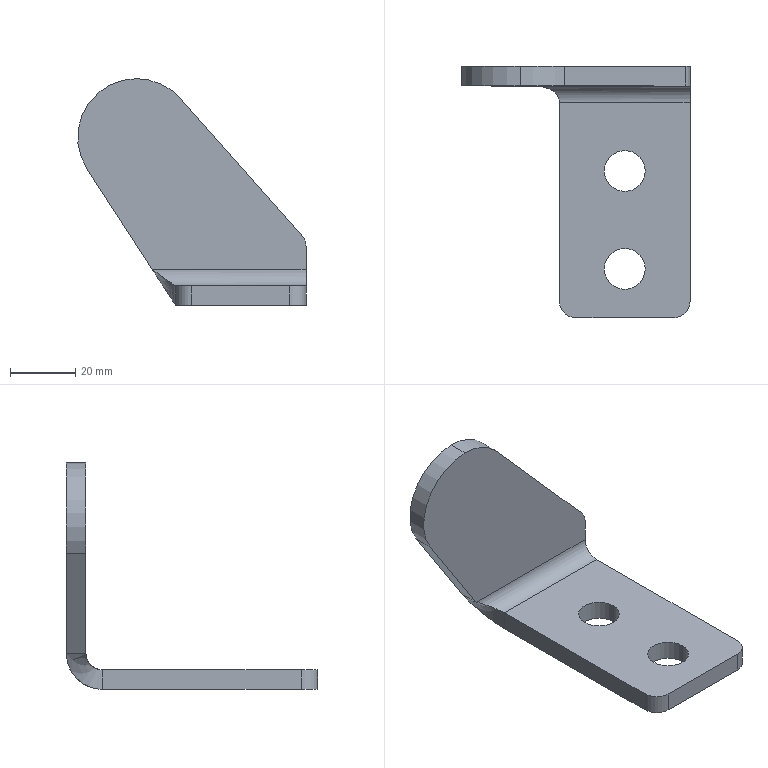Part | SolidWorks | features ICE 2, Fillet 1, FlatPattern 1, SMBaseFlange 1, SheetMetal 1 | 1 solid | 23 faces | box 70 x 77 x 69.5 mm | volume 32666 mm3 | cylinder 11 | plane 11 | spline 1 | commonest cylinder face diameters 10 x4 12.5 x4 36 x2 22 x1
STEP:
#1=CARTESIAN_POINT('',(-52.,71.,69.5));
#2=VERTEX_POINT('',#1);
#3=CARTESIAN_POINT('',(-67.093,71.,41.692));
#4=VERTEX_POINT('',#3);
#5=CARTESIAN_POINT('',(-52.,71.,51.5));
#6=DIRECTION('',(0.,-1.,0.));
#7=DIRECTION('',(0.,0.,1.));
#8=AXIS2_PLACEMENT_3D('',#5,#6,#7);
#9=CIRCLE('',#8,18.);
#10=EDGE_CURVE('',#2,#4,#9,.T.);
#11=ORIENTED_EDGE('',*,*,#10,.F.);
#12=CARTESIAN_POINT('',(-52.,77.,69.5));
#13=VERTEX_POINT('',#12);
#14=CARTESIAN_POINT('',(-52.,71.,69.5));
#15=DIRECTION('',(0.,1.,0.));
#16=VECTOR('',#15,1000.);
#17=LINE('',#14,#16);
#18=EDGE_CURVE('',#2,#13,#17,.T.);
#19=ORIENTED_EDGE('',*,*,#18,.T.);
#20=CARTESIAN_POINT('',(-67.093,77.,41.692));
#21=VERTEX_POINT('',#20);
#22=CARTESIAN_POINT('',(-52.,77.,51.5));
#23=DIRECTION('',(0.,-1.,0.));
#24=DIRECTION('',(0.,0.,1.));
#25=AXIS2_PLACEMENT_3D('',#22,#23,#24);
#26=CIRCLE('',#25,18.);
#27=EDGE_CURVE('',#13,#21,#26,.T.);
#28=ORIENTED_EDGE('',*,*,#27,.T.);
#29=CARTESIAN_POINT('',(-67.093,71.,41.692));
#30=DIRECTION('',(0.,1.,0.));
#31=VECTOR('',#30,1000.);
#32=LINE('',#29,#31);
#33=EDGE_CURVE('',#4,#21,#32,.T.);
#34=ORIENTED_EDGE('',*,*,#33,.F.);
#35=EDGE_LOOP('',(#11,#19,#28,#34));
#36=FACE_OUTER_BOUND('',#35,.T.);
#37=CARTESIAN_POINT('',(-52.,71.,51.5));
#38=DIRECTION('',(0.,1.,0.));
#39=DIRECTION('',(0.,0.,1.));
#40=AXIS2_PLACEMENT_3D('',#37,#38,#39);
#41=CYLINDRICAL_SURFACE('',#40,18.);
#42=ADVANCED_FACE('',(#36),#41,.T.);
#43=CARTESIAN_POINT('',(-26.25,15.,0.));
#44=VERTEX_POINT('',#43);
#45=CARTESIAN_POINT('',(-13.75,15.,0.));
#46=VERTEX_POINT('',#45);
#47=CARTESIAN_POINT('',(-20.,15.,0.));
#48=DIRECTION('',(0.,0.,1.));
#49=DIRECTION('',(-1.,0.,0.));
#50=AXIS2_PLACEMENT_3D('',#47,#48,#49);
#51=CIRCLE('',#50,6.25);
#52=EDGE_CURVE('',#44,#46,#51,.T.);
#53=ORIENTED_EDGE('',*,*,#52,.F.);
#54=CARTESIAN_POINT('',(-26.25,15.,6.));
#55=VERTEX_POINT('',#54);
#56=CARTESIAN_POINT('',(-26.25,15.,-0.001));
#57=DIRECTION('',(0.,0.,1.));
#58=VECTOR('',#57,1000.);
#59=LINE('',#56,#58);
#60=EDGE_CURVE('',#44,#55,#59,.T.);
#61=ORIENTED_EDGE('',*,*,#60,.T.);
#62=CARTESIAN_POINT('',(-13.75,15.,6.));
#63=VERTEX_POINT('',#62);
#64=CARTESIAN_POINT('',(-20.,15.,6.));
#65=DIRECTION('',(0.,0.,1.));
#66=DIRECTION('',(1.,0.,0.));
#67=AXIS2_PLACEMENT_3D('',#64,#65,#66);
#68=CIRCLE('',#67,6.25);
#69=EDGE_CURVE('',#55,#63,#68,.T.);
#70=ORIENTED_EDGE('',*,*,#69,.T.);
#71=CARTESIAN_POINT('',(-13.75,15.,-0.001));
#72=DIRECTION('',(0.,0.,1.));
#73=VECTOR('',#72,1000.);
#74=LINE('',#71,#73);
#75=EDGE_CURVE('',#46,#63,#74,.T.);
#76=ORIENTED_EDGE('',*,*,#75,.F.);
#77=EDGE_LOOP('',(#53,#61,#70,#76));
#78=FACE_OUTER_BOUND('',#77,.T.);
#79=CARTESIAN_POINT('',(-20.,15.,-0.001));
#80=DIRECTION('',(0.,0.,1.));
#81=DIRECTION('',(1.,0.,0.));
#82=AXIS2_PLACEMENT_3D('',#79,#80,#81);
#83=CYLINDRICAL_SURFACE('',#82,6.25);
#84=ADVANCED_FACE('',(#78),#83,.F.);
#85=CARTESIAN_POINT('',(-26.25,45.,0.));
#86=VERTEX_POINT('',#85);
#87=CARTESIAN_POINT('',(-13.75,45.,0.));
#88=VERTEX_POINT('',#87);
#89=CARTESIAN_POINT('',(-20.,45.,0.));
#90=DIRECTION('',(0.,0.,1.));
#91=DIRECTION('',(-1.,0.,0.));
#92=AXIS2_PLACEMENT_3D('',#89,#90,#91);
#93=CIRCLE('',#92,6.25);
#94=EDGE_CURVE('',#86,#88,#93,.T.);
#95=ORIENTED_EDGE('',*,*,#94,.F.);
#96=CARTESIAN_POINT('',(-26.25,45.,6.));
#97=VERTEX_POINT('',#96);
#98=CARTESIAN_POINT('',(-26.25,45.,-0.001));
#99=DIRECTION('',(0.,0.,1.));
#100=VECTOR('',#99,1000.);
#101=LINE('',#98,#100);
#102=EDGE_CURVE('',#86,#97,#101,.T.);
#103=ORIENTED_EDGE('',*,*,#102,.T.);
#104=CARTESIAN_POINT('',(-13.75,45.,6.));
#105=VERTEX_POINT('',#104);
#106=CARTESIAN_POINT('',(-20.,45.,6.));
#107=DIRECTION('',(0.,0.,1.));
#108=DIRECTION('',(1.,0.,0.));
#109=AXIS2_PLACEMENT_3D('',#106,#107,#108);
#110=CIRCLE('',#109,6.25);
#111=EDGE_CURVE('',#97,#105,#110,.T.);
#112=ORIENTED_EDGE('',*,*,#111,.T.);
#113=CARTESIAN_POINT('',(-13.75,45.,-0.001));
#114=DIRECTION('',(0.,0.,1.));
#115=VECTOR('',#114,1000.);
#116=LINE('',#113,#115);
#117=EDGE_CURVE('',#88,#105,#116,.T.);
#118=ORIENTED_EDGE('',*,*,#117,.F.);
#119=EDGE_LOOP('',(#95,#103,#112,#118));
#120=FACE_OUTER_BOUND('',#119,.T.);
#121=CARTESIAN_POINT('',(-20.,45.,-0.001));
#122=DIRECTION('',(0.,0.,1.));
#123=DIRECTION('',(1.,0.,0.));
#124=AXIS2_PLACEMENT_3D('',#121,#122,#123);
#125=CYLINDRICAL_SURFACE('',#124,6.25);
#126=ADVANCED_FACE('',(#120),#125,.F.);
#127=CARTESIAN_POINT('',(-38.534,77.,63.444));
#128=VERTEX_POINT('',#127);
#129=CARTESIAN_POINT('',(-1.259,77.,21.42));
#130=VERTEX_POINT('',#129);
#131=CARTESIAN_POINT('',(9.929,77.,8.806));
#132=DIRECTION('',(0.6636,0.,-0.7481));
#133=VECTOR('',#132,1000.);
#134=LINE('',#131,#133);
#135=EDGE_CURVE('',#128,#130,#134,.T.);
#136=ORIENTED_EDGE('',*,*,#135,.T.);
#137=CARTESIAN_POINT('',(0.,77.,18.102));
#138=VERTEX_POINT('',#137);
#139=CARTESIAN_POINT('',(-5.,77.,18.102));
#140=DIRECTION('',(0.,1.,0.));
#141=DIRECTION('',(0.,0.,1.));
#142=AXIS2_PLACEMENT_3D('',#139,#140,#141);
#143=CIRCLE('',#142,5.);
#144=EDGE_CURVE('',#130,#138,#143,.T.);
#145=ORIENTED_EDGE('',*,*,#144,.T.);
#146=CARTESIAN_POINT('',(0.,77.,11.));
#147=VERTEX_POINT('',#146);
#148=CARTESIAN_POINT('',(0.,77.,0.));
#149=DIRECTION('',(0.,0.,1.));
#150=VECTOR('',#149,1000.);
#151=LINE('',#148,#150);
#152=EDGE_CURVE('',#147,#138,#151,.T.);
#153=ORIENTED_EDGE('',*,*,#152,.F.);
#154=CARTESIAN_POINT('',(-47.148,77.,11.));
#155=VERTEX_POINT('',#154);
#156=CARTESIAN_POINT('',(-70.,77.,11.));
#157=DIRECTION('',(1.,0.,0.));
#158=VECTOR('',#157,1000.);
#159=LINE('',#156,#158);
#160=EDGE_CURVE('',#155,#147,#159,.T.);
#161=ORIENTED_EDGE('',*,*,#160,.F.);
#162=CARTESIAN_POINT('',(-28.124,77.,-18.276));
#163=DIRECTION('',(-0.5449,0.,0.8385));
#164=VECTOR('',#163,1000.);
#165=LINE('',#162,#164);
#166=EDGE_CURVE('',#155,#21,#165,.T.);
#167=ORIENTED_EDGE('',*,*,#166,.T.);
#168=ORIENTED_EDGE('',*,*,#27,.F.);
#169=CARTESIAN_POINT('',(-52.,77.,51.5));
#170=DIRECTION('',(0.,-1.,0.));
#171=DIRECTION('',(0.,0.,1.));
#172=AXIS2_PLACEMENT_3D('',#169,#170,#171);
#173=CIRCLE('',#172,18.);
#174=EDGE_CURVE('',#128,#13,#173,.T.);
#175=ORIENTED_EDGE('',*,*,#174,.F.);
#176=EDGE_LOOP('',(#136,#145,#153,#161,#167,#168,#175));
#177=FACE_OUTER_BOUND('',#176,.T.);
#178=CARTESIAN_POINT('',(-70.,77.,0.));
#179=DIRECTION('',(0.,1.,0.));
#180=DIRECTION('',(0.,0.,1.));
#181=AXIS2_PLACEMENT_3D('',#178,#179,#180);
#182=PLANE('',#181);
#183=ADVANCED_FACE('',(#177),#182,.T.);
#184=CARTESIAN_POINT('',(0.,71.,11.));
#185=VERTEX_POINT('',#184);
#186=CARTESIAN_POINT('',(0.,71.,18.102));
#187=VERTEX_POINT('',#186);
#188=CARTESIAN_POINT('',(0.,71.,0.));
#189=DIRECTION('',(0.,0.,1.));
#190=VECTOR('',#189,1000.);
#191=LINE('',#188,#190);
#192=EDGE_CURVE('',#185,#187,#191,.T.);
#193=ORIENTED_EDGE('',*,*,#192,.T.);
#194=CARTESIAN_POINT('',(-1.259,71.,21.42));
#195=VERTEX_POINT('',#194);
#196=CARTESIAN_POINT('',(-5.,71.,18.102));
#197=DIRECTION('',(0.,-1.,0.));
#198=DIRECTION('',(0.,0.,1.));
#199=AXIS2_PLACEMENT_3D('',#196,#197,#198);
#200=CIRCLE('',#199,5.);
#201=EDGE_CURVE('',#187,#195,#200,.T.);
#202=ORIENTED_EDGE('',*,*,#201,.T.);
#203=CARTESIAN_POINT('',(-38.534,71.,63.444));
#204=VERTEX_POINT('',#203);
#205=CARTESIAN_POINT('',(9.929,71.,8.806));
#206=DIRECTION('',(0.6636,0.,-0.7481));
#207=VECTOR('',#206,1000.);
#208=LINE('',#205,#207);
#209=EDGE_CURVE('',#204,#195,#208,.T.);
#210=ORIENTED_EDGE('',*,*,#209,.F.);
#211=CARTESIAN_POINT('',(-52.,71.,51.5));
#212=DIRECTION('',(0.,-1.,0.));
#213=DIRECTION('',(0.,0.,1.));
#214=AXIS2_PLACEMENT_3D('',#211,#212,#213);
#215=CIRCLE('',#214,18.);
#216=EDGE_CURVE('',#204,#2,#215,.T.);
#217=ORIENTED_EDGE('',*,*,#216,.T.);
#218=ORIENTED_EDGE('',*,*,#10,.T.);
#219=CARTESIAN_POINT('',(-47.148,71.,11.));
#220=VERTEX_POINT('',#219);
#221=CARTESIAN_POINT('',(-28.124,71.,-18.276));
#222=DIRECTION('',(-0.5449,0.,0.8385));
#223=VECTOR('',#222,1000.);
#224=LINE('',#221,#223);
#225=EDGE_CURVE('',#220,#4,#224,.T.);
#226=ORIENTED_EDGE('',*,*,#225,.F.);
#227=CARTESIAN_POINT('',(-70.,71.,11.));
#228=DIRECTION('',(1.,0.,0.));
#229=VECTOR('',#228,1000.);
#230=LINE('',#227,#229);
#231=EDGE_CURVE('',#220,#185,#230,.T.);
#232=ORIENTED_EDGE('',*,*,#231,.T.);
#233=EDGE_LOOP('',(#193,#202,#210,#217,#218,#226,#232));
#234=FACE_OUTER_BOUND('',#233,.T.);
#235=CARTESIAN_POINT('',(-70.,71.,0.));
#236=DIRECTION('',(0.,1.,0.));
#237=DIRECTION('',(0.,0.,1.));
#238=AXIS2_PLACEMENT_3D('',#235,#236,#237);
#239=PLANE('',#238);
#240=ADVANCED_FACE('',(#234),#239,.F.);
#241=CARTESIAN_POINT('',(-40.,66.,0.));
#242=VERTEX_POINT('',#241);
#243=CARTESIAN_POINT('',(0.,66.,0.));
#244=VERTEX_POINT('',#243);
#245=CARTESIAN_POINT('',(-70.,66.,0.));
#246=DIRECTION('',(1.,0.,0.));
#247=VECTOR('',#246,1000.);
#248=LINE('',#245,#247);
#249=EDGE_CURVE('',#242,#244,#248,.T.);
#250=ORIENTED_EDGE('',*,*,#249,.F.);
#251=CARTESIAN_POINT('',(-40.,66.,0.));
#252=CARTESIAN_POINT('',(-40.,72.444,0.));
#253=CARTESIAN_POINT('',(-42.961,77.,4.556));
#254=CARTESIAN_POINT('',(-47.148,77.,11.));
#255=(BOUNDED_CURVE()B_SPLINE_CURVE(3,(#251,#252,#253,#254),.UNSPECIFIED.,.F.,.F.)B_SPLINE_CURVE_WITH_KNOTS((4,4),(0.,1.571),.UNSPECIFIED.)CURVE()GEOMETRIC_REPRESENTATION_ITEM()RATIONAL_B_SPLINE_CURVE((1.,0.8047,0.8047,1.))REPRESENTATION_ITEM(''));
#256=EDGE_CURVE('',#242,#155,#255,.T.);
#257=ORIENTED_EDGE('',*,*,#256,.T.);
#258=ORIENTED_EDGE('',*,*,#160,.T.);
#259=CARTESIAN_POINT('',(0.,66.,11.));
#260=DIRECTION('',(1.,0.,0.));
#261=DIRECTION('',(0.,0.,1.));
#262=AXIS2_PLACEMENT_3D('',#259,#260,#261);
#263=CIRCLE('',#262,11.);
#264=EDGE_CURVE('',#244,#147,#263,.T.);
#265=ORIENTED_EDGE('',*,*,#264,.F.);
#266=EDGE_LOOP('',(#250,#257,#258,#265));
#267=FACE_OUTER_BOUND('',#266,.T.);
#268=CARTESIAN_POINT('',(-70.,66.,11.));
#269=DIRECTION('',(1.,0.,0.));
#270=DIRECTION('',(0.,0.,-1.));
#271=AXIS2_PLACEMENT_3D('',#268,#269,#270);
#272=CYLINDRICAL_SURFACE('',#271,11.);
#273=ADVANCED_FACE('',(#267),#272,.T.);
#274=CARTESIAN_POINT('',(-20.,15.,0.));
#275=DIRECTION('',(0.,0.,1.));
#276=DIRECTION('',(-1.,0.,0.));
#277=AXIS2_PLACEMENT_3D('',#274,#275,#276);
#278=CIRCLE('',#277,6.25);
#279=EDGE_CURVE('',#46,#44,#278,.T.);
#280=ORIENTED_EDGE('',*,*,#279,.T.);
#281=ORIENTED_EDGE('',*,*,#52,.T.);
#282=EDGE_LOOP('',(#280,#281));
#283=FACE_BOUND('',#282,.T.);
#284=CARTESIAN_POINT('',(-20.,45.,0.));
#285=DIRECTION('',(0.,0.,1.));
#286=DIRECTION('',(-1.,0.,0.));
#287=AXIS2_PLACEMENT_3D('',#284,#285,#286);
#288=CIRCLE('',#287,6.25);
#289=EDGE_CURVE('',#88,#86,#288,.T.);
#290=ORIENTED_EDGE('',*,*,#289,.T.);
#291=ORIENTED_EDGE('',*,*,#94,.T.);
#292=EDGE_LOOP('',(#290,#291));
#293=FACE_BOUND('',#292,.T.);
#294=CARTESIAN_POINT('',(0.,5.,0.));
#295=VERTEX_POINT('',#294);
#296=CARTESIAN_POINT('',(0.,0.,0.));
#297=DIRECTION('',(0.,1.,0.));
#298=VECTOR('',#297,1000.);
#299=LINE('',#296,#298);
#300=EDGE_CURVE('',#295,#244,#299,.T.);
#301=ORIENTED_EDGE('',*,*,#300,.F.);
#302=CARTESIAN_POINT('',(-5.,0.,0.));
#303=VERTEX_POINT('',#302);
#304=CARTESIAN_POINT('',(-5.,5.,0.));
#305=DIRECTION('',(0.,0.,-1.));
#306=DIRECTION('',(-1.,0.,0.));
#307=AXIS2_PLACEMENT_3D('',#304,#305,#306);
#308=CIRCLE('',#307,5.);
#309=EDGE_CURVE('',#295,#303,#308,.T.);
#310=ORIENTED_EDGE('',*,*,#309,.T.);
#311=CARTESIAN_POINT('',(-35.,0.,0.));
#312=VERTEX_POINT('',#311);
#313=CARTESIAN_POINT('',(-70.,0.,0.));
#314=DIRECTION('',(1.,0.,0.));
#315=VECTOR('',#314,1000.);
#316=LINE('',#313,#315);
#317=EDGE_CURVE('',#312,#303,#316,.T.);
#318=ORIENTED_EDGE('',*,*,#317,.F.);
#319=CARTESIAN_POINT('',(-40.,5.,0.));
#320=VERTEX_POINT('',#319);
#321=CARTESIAN_POINT('',(-35.,5.,0.));
#322=DIRECTION('',(0.,0.,-1.));
#323=DIRECTION('',(-1.,0.,0.));
#324=AXIS2_PLACEMENT_3D('',#321,#322,#323);
#325=CIRCLE('',#324,5.);
#326=EDGE_CURVE('',#312,#320,#325,.T.);
#327=ORIENTED_EDGE('',*,*,#326,.T.);
#328=CARTESIAN_POINT('',(-40.,-0.001,0.));
#329=DIRECTION('',(0.,1.,0.));
#330=VECTOR('',#329,1000.);
#331=LINE('',#328,#330);
#332=EDGE_CURVE('',#320,#242,#331,.T.);
#333=ORIENTED_EDGE('',*,*,#332,.T.);
#334=ORIENTED_EDGE('',*,*,#249,.T.);
#335=EDGE_LOOP('',(#301,#310,#318,#327,#333,#334));
#336=FACE_OUTER_BOUND('',#335,.T.);
#337=CARTESIAN_POINT('',(-70.,0.,0.));
#338=DIRECTION('',(0.,0.,-1.));
#339=DIRECTION('',(-1.,0.,0.));
#340=AXIS2_PLACEMENT_3D('',#337,#338,#339);
#341=PLANE('',#340);
#342=ADVANCED_FACE('',(#283,#293,#336),#341,.T.);
#343=ORIENTED_EDGE('',*,*,#317,.T.);
#344=CARTESIAN_POINT('',(-5.,0.,6.));
#345=VERTEX_POINT('',#344);
#346=CARTESIAN_POINT('',(-5.,0.,6.));
#347=DIRECTION('',(0.,0.,1.));
#348=VECTOR('',#347,1000.);
#349=LINE('',#346,#348);
#350=EDGE_CURVE('',#303,#345,#349,.T.);
#351=ORIENTED_EDGE('',*,*,#350,.T.);
#352=CARTESIAN_POINT('',(-35.,0.,6.));
#353=VERTEX_POINT('',#352);
#354=CARTESIAN_POINT('',(-70.,0.,6.));
#355=DIRECTION('',(1.,0.,0.));
#356=VECTOR('',#355,1000.);
#357=LINE('',#354,#356);
#358=EDGE_CURVE('',#353,#345,#357,.T.);
#359=ORIENTED_EDGE('',*,*,#358,.F.);
#360=CARTESIAN_POINT('',(-35.,0.,0.));
#361=DIRECTION('',(0.,0.,-1.));
#362=VECTOR('',#361,1000.);
#363=LINE('',#360,#362);
#364=EDGE_CURVE('',#353,#312,#363,.T.);
#365=ORIENTED_EDGE('',*,*,#364,.T.);
#366=EDGE_LOOP('',(#343,#351,#359,#365));
#367=FACE_OUTER_BOUND('',#366,.T.);
#368=CARTESIAN_POINT('',(-70.,0.,0.));
#369=DIRECTION('',(0.,1.,0.));
#370=DIRECTION('',(0.,0.,1.));
#371=AXIS2_PLACEMENT_3D('',#368,#369,#370);
#372=PLANE('',#371);
#373=ADVANCED_FACE('',(#367),#372,.F.);
#374=CARTESIAN_POINT('',(-20.,45.,6.));
#375=DIRECTION('',(0.,0.,1.));
#376=DIRECTION('',(1.,0.,0.));
#377=AXIS2_PLACEMENT_3D('',#374,#375,#376);
#378=CIRCLE('',#377,6.25);
#379=EDGE_CURVE('',#105,#97,#378,.T.);
#380=ORIENTED_EDGE('',*,*,#379,.F.);
#381=ORIENTED_EDGE('',*,*,#111,.F.);
#382=EDGE_LOOP('',(#380,#381));
#383=FACE_BOUND('',#382,.T.);
#384=CARTESIAN_POINT('',(-20.,15.,6.));
#385=DIRECTION('',(0.,0.,1.));
#386=DIRECTION('',(1.,0.,0.));
#387=AXIS2_PLACEMENT_3D('',#384,#385,#386);
#388=CIRCLE('',#387,6.25);
#389=EDGE_CURVE('',#63,#55,#388,.T.);
#390=ORIENTED_EDGE('',*,*,#389,.F.);
#391=ORIENTED_EDGE('',*,*,#69,.F.);
#392=EDGE_LOOP('',(#390,#391));
#393=FACE_BOUND('',#392,.T.);
#394=ORIENTED_EDGE('',*,*,#358,.T.);
#395=CARTESIAN_POINT('',(0.,5.,6.));
#396=VERTEX_POINT('',#395);
#397=CARTESIAN_POINT('',(-5.,5.,6.));
#398=DIRECTION('',(0.,0.,1.));
#399=DIRECTION('',(-1.,0.,0.));
#400=AXIS2_PLACEMENT_3D('',#397,#398,#399);
#401=CIRCLE('',#400,5.);
#402=EDGE_CURVE('',#345,#396,#401,.T.);
#403=ORIENTED_EDGE('',*,*,#402,.T.);
#404=CARTESIAN_POINT('',(0.,66.,6.));
#405=VERTEX_POINT('',#404);
#406=CARTESIAN_POINT('',(0.,0.,6.));
#407=DIRECTION('',(0.,1.,0.));
#408=VECTOR('',#407,1000.);
#409=LINE('',#406,#408);
#410=EDGE_CURVE('',#396,#405,#409,.T.);
#411=ORIENTED_EDGE('',*,*,#410,.T.);
#412=CARTESIAN_POINT('',(-40.,66.,6.));
#413=VERTEX_POINT('',#412);
#414=CARTESIAN_POINT('',(-70.,66.,6.));
#415=DIRECTION('',(1.,0.,0.));
#416=VECTOR('',#415,1000.);
#417=LINE('',#414,#416);
#418=EDGE_CURVE('',#413,#405,#417,.T.);
#419=ORIENTED_EDGE('',*,*,#418,.F.);
#420=CARTESIAN_POINT('',(-40.,5.,6.));
#421=VERTEX_POINT('',#420);
#422=CARTESIAN_POINT('',(-40.,0.,6.));
#423=DIRECTION('',(0.,1.,0.));
#424=VECTOR('',#423,1000.);
#425=LINE('',#422,#424);
#426=EDGE_CURVE('',#421,#413,#425,.T.);
#427=ORIENTED_EDGE('',*,*,#426,.F.);
#428=CARTESIAN_POINT('',(-35.,5.,6.));
#429=DIRECTION('',(0.,0.,1.));
#430=DIRECTION('',(-1.,0.,0.));
#431=AXIS2_PLACEMENT_3D('',#428,#429,#430);
#432=CIRCLE('',#431,5.);
#433=EDGE_CURVE('',#421,#353,#432,.T.);
#434=ORIENTED_EDGE('',*,*,#433,.T.);
#435=EDGE_LOOP('',(#394,#403,#411,#419,#427,#434));
#436=FACE_OUTER_BOUND('',#435,.T.);
#437=CARTESIAN_POINT('',(-70.,0.,6.));
#438=DIRECTION('',(0.,0.,-1.));
#439=DIRECTION('',(-1.,0.,0.));
#440=AXIS2_PLACEMENT_3D('',#437,#438,#439);
#441=PLANE('',#440);
#442=ADVANCED_FACE('',(#383,#393,#436),#441,.F.);
#443=CARTESIAN_POINT('',(-40.,66.,6.));
#444=CARTESIAN_POINT('',(-40.,68.929,6.));
#445=CARTESIAN_POINT('',(-42.961,71.,8.071));
#446=CARTESIAN_POINT('',(-47.148,71.,11.));
#447=(BOUNDED_CURVE()B_SPLINE_CURVE(3,(#443,#444,#445,#446),.UNSPECIFIED.,.F.,.F.)B_SPLINE_CURVE_WITH_KNOTS((4,4),(0.,1.571),.UNSPECIFIED.)CURVE()GEOMETRIC_REPRESENTATION_ITEM()RATIONAL_B_SPLINE_CURVE((1.,0.8047,0.8047,1.))REPRESENTATION_ITEM(''));
#448=EDGE_CURVE('',#413,#220,#447,.T.);
#449=ORIENTED_EDGE('',*,*,#448,.F.);
#450=ORIENTED_EDGE('',*,*,#418,.T.);
#451=CARTESIAN_POINT('',(0.,66.,11.));
#452=DIRECTION('',(1.,0.,0.));
#453=DIRECTION('',(0.,0.,-1.));
#454=AXIS2_PLACEMENT_3D('',#451,#452,#453);
#455=CIRCLE('',#454,5.);
#456=EDGE_CURVE('',#405,#185,#455,.T.);
#457=ORIENTED_EDGE('',*,*,#456,.T.);
#458=ORIENTED_EDGE('',*,*,#231,.F.);
#459=EDGE_LOOP('',(#449,#450,#457,#458));
#460=FACE_OUTER_BOUND('',#459,.T.);
#461=CARTESIAN_POINT('',(-70.,66.,11.));
#462=DIRECTION('',(1.,0.,0.));
#463=DIRECTION('',(0.,0.,-1.));
#464=AXIS2_PLACEMENT_3D('',#461,#462,#463);
#465=CYLINDRICAL_SURFACE('',#464,5.);
#466=ADVANCED_FACE('',(#460),#465,.F.);
#467=ORIENTED_EDGE('',*,*,#152,.T.);
#468=CARTESIAN_POINT('',(0.,66.,18.102));
#469=DIRECTION('',(0.,-1.,0.));
#470=VECTOR('',#469,1000.);
#471=LINE('',#468,#470);
#472=EDGE_CURVE('',#138,#187,#471,.T.);
#473=ORIENTED_EDGE('',*,*,#472,.T.);
#474=ORIENTED_EDGE('',*,*,#192,.F.);
#475=CARTESIAN_POINT('',(0.,71.,11.));
#476=DIRECTION('',(0.,1.,0.));
#477=VECTOR('',#476,1000.);
#478=LINE('',#475,#477);
#479=EDGE_CURVE('',#185,#147,#478,.T.);
#480=ORIENTED_EDGE('',*,*,#479,.T.);
#481=EDGE_LOOP('',(#467,#473,#474,#480));
#482=FACE_OUTER_BOUND('',#481,.T.);
#483=CARTESIAN_POINT('',(0.,66.,11.));
#484=DIRECTION('',(1.,0.,0.));
#485=DIRECTION('',(0.,0.,-1.));
#486=AXIS2_PLACEMENT_3D('',#483,#484,#485);
#487=PLANE('',#486);
#488=ADVANCED_FACE('',(#482),#487,.T.);
#489=CARTESIAN_POINT('',(0.,66.,0.));
#490=DIRECTION('',(0.,0.,1.));
#491=VECTOR('',#490,1000.);
#492=LINE('',#489,#491);
#493=EDGE_CURVE('',#244,#405,#492,.T.);
#494=ORIENTED_EDGE('',*,*,#493,.F.);
#495=ORIENTED_EDGE('',*,*,#264,.T.);
#496=ORIENTED_EDGE('',*,*,#479,.F.);
#497=ORIENTED_EDGE('',*,*,#456,.F.);
#498=EDGE_LOOP('',(#494,#495,#496,#497));
#499=FACE_OUTER_BOUND('',#498,.T.);
#500=CARTESIAN_POINT('',(0.,66.,0.));
#501=DIRECTION('',(1.,0.,0.));
#502=DIRECTION('',(0.,0.,-1.));
#503=AXIS2_PLACEMENT_3D('',#500,#501,#502);
#504=PLANE('',#503);
#505=ADVANCED_FACE('',(#499),#504,.T.);
#506=ORIENTED_EDGE('',*,*,#410,.F.);
#507=CARTESIAN_POINT('',(0.,5.,0.));
#508=DIRECTION('',(0.,0.,-1.));
#509=VECTOR('',#508,1000.);
#510=LINE('',#507,#509);
#511=EDGE_CURVE('',#396,#295,#510,.T.);
#512=ORIENTED_EDGE('',*,*,#511,.T.);
#513=ORIENTED_EDGE('',*,*,#300,.T.);
#514=ORIENTED_EDGE('',*,*,#493,.T.);
#515=EDGE_LOOP('',(#506,#512,#513,#514));
#516=FACE_OUTER_BOUND('',#515,.T.);
#517=CARTESIAN_POINT('',(0.,71.,11.));
#518=DIRECTION('',(1.,0.,0.));
#519=DIRECTION('',(0.,0.,-1.));
#520=AXIS2_PLACEMENT_3D('',#517,#518,#519);
#521=PLANE('',#520);
#522=ADVANCED_FACE('',(#516),#521,.T.);
#523=ORIENTED_EDGE('',*,*,#102,.F.);
#524=ORIENTED_EDGE('',*,*,#289,.F.);
#525=ORIENTED_EDGE('',*,*,#117,.T.);
#526=ORIENTED_EDGE('',*,*,#379,.T.);
#527=EDGE_LOOP('',(#523,#524,#525,#526));
#528=FACE_OUTER_BOUND('',#527,.T.);
#529=CARTESIAN_POINT('',(-20.,45.,-0.001));
#530=DIRECTION('',(0.,0.,1.));
#531=DIRECTION('',(1.,0.,0.));
#532=AXIS2_PLACEMENT_3D('',#529,#530,#531);
#533=CYLINDRICAL_SURFACE('',#532,6.25);
#534=ADVANCED_FACE('',(#528),#533,.F.);
#535=ORIENTED_EDGE('',*,*,#60,.F.);
#536=ORIENTED_EDGE('',*,*,#279,.F.);
#537=ORIENTED_EDGE('',*,*,#75,.T.);
#538=ORIENTED_EDGE('',*,*,#389,.T.);
#539=EDGE_LOOP('',(#535,#536,#537,#538));
#540=FACE_OUTER_BOUND('',#539,.T.);
#541=CARTESIAN_POINT('',(-20.,15.,-0.001));
#542=DIRECTION('',(0.,0.,1.));
#543=DIRECTION('',(1.,0.,0.));
#544=AXIS2_PLACEMENT_3D('',#541,#542,#543);
#545=CYLINDRICAL_SURFACE('',#544,6.25);
#546=ADVANCED_FACE('',(#540),#545,.F.);
#547=ORIENTED_EDGE('',*,*,#18,.F.);
#548=ORIENTED_EDGE('',*,*,#216,.F.);
#549=CARTESIAN_POINT('',(-38.534,71.,63.444));
#550=DIRECTION('',(0.,1.,0.));
#551=VECTOR('',#550,1000.);
#552=LINE('',#549,#551);
#553=EDGE_CURVE('',#204,#128,#552,.T.);
#554=ORIENTED_EDGE('',*,*,#553,.T.);
#555=ORIENTED_EDGE('',*,*,#174,.T.);
#556=EDGE_LOOP('',(#547,#548,#554,#555));
#557=FACE_OUTER_BOUND('',#556,.T.);
#558=CARTESIAN_POINT('',(-52.,71.,51.5));
#559=DIRECTION('',(0.,1.,0.));
#560=DIRECTION('',(0.,0.,1.));
#561=AXIS2_PLACEMENT_3D('',#558,#559,#560);
#562=CYLINDRICAL_SURFACE('',#561,18.);
#563=ADVANCED_FACE('',(#557),#562,.T.);
#564=CARTESIAN_POINT('',(-47.148,71.,11.));
#565=DIRECTION('',(0.,1.,0.));
#566=VECTOR('',#565,1000.);
#567=LINE('',#564,#566);
#568=EDGE_CURVE('',#220,#155,#567,.T.);
#569=ORIENTED_EDGE('',*,*,#568,.F.);
#570=ORIENTED_EDGE('',*,*,#225,.T.);
#571=ORIENTED_EDGE('',*,*,#33,.T.);
#572=ORIENTED_EDGE('',*,*,#166,.F.);
#573=EDGE_LOOP('',(#569,#570,#571,#572));
#574=FACE_OUTER_BOUND('',#573,.T.);
#575=CARTESIAN_POINT('',(-28.124,71.,-18.276));
#576=DIRECTION('',(-0.8385,0.,-0.5449));
#577=DIRECTION('',(-0.5449,0.,0.8385));
#578=AXIS2_PLACEMENT_3D('',#575,#576,#577);
#579=PLANE('',#578);
#580=ADVANCED_FACE('',(#574),#579,.T.);
#581=ORIENTED_EDGE('',*,*,#332,.F.);
#582=CARTESIAN_POINT('',(-40.,5.,6.));
#583=DIRECTION('',(0.,0.,1.));
#584=VECTOR('',#583,1000.);
#585=LINE('',#582,#584);
#586=EDGE_CURVE('',#320,#421,#585,.T.);
#587=ORIENTED_EDGE('',*,*,#586,.T.);
#588=ORIENTED_EDGE('',*,*,#426,.T.);
#589=CARTESIAN_POINT('',(-40.,66.,0.));
#590=DIRECTION('',(0.,0.,1.));
#591=VECTOR('',#590,1000.);
#592=LINE('',#589,#591);
#593=EDGE_CURVE('',#242,#413,#592,.T.);
#594=ORIENTED_EDGE('',*,*,#593,.F.);
#595=EDGE_LOOP('',(#581,#587,#588,#594));
#596=FACE_OUTER_BOUND('',#595,.T.);
#597=CARTESIAN_POINT('',(-40.,-0.001,0.));
#598=DIRECTION('',(-1.,0.,0.));
#599=DIRECTION('',(0.,1.,0.));
#600=AXIS2_PLACEMENT_3D('',#597,#598,#599);
#601=PLANE('',#600);
#602=ADVANCED_FACE('',(#596),#601,.T.);
#603=ORIENTED_EDGE('',*,*,#256,.F.);
#604=ORIENTED_EDGE('',*,*,#593,.T.);
#605=ORIENTED_EDGE('',*,*,#448,.T.);
#606=ORIENTED_EDGE('',*,*,#568,.T.);
#607=EDGE_LOOP('',(#603,#604,#605,#606));
#608=FACE_OUTER_BOUND('',#607,.T.);
#609=CARTESIAN_POINT('',(-40.,66.,6.));
#610=CARTESIAN_POINT('',(-40.,66.,4.));
#611=CARTESIAN_POINT('',(-40.,66.,2.));
#612=CARTESIAN_POINT('',(-40.,66.,0.));
#613=CARTESIAN_POINT('',(-40.,76.,6.));
#614=CARTESIAN_POINT('',(-40.,80.,4.));
#615=CARTESIAN_POINT('',(-40.,84.,2.));
#616=CARTESIAN_POINT('',(-40.,88.,0.));
#617=CARTESIAN_POINT('',(-54.296,76.,16.));
#618=CARTESIAN_POINT('',(-54.296,80.,18.));
#619=CARTESIAN_POINT('',(-54.296,84.,20.));
#620=CARTESIAN_POINT('',(-54.296,88.,22.));
#621=CARTESIAN_POINT('',(-54.296,66.,16.));
#622=CARTESIAN_POINT('',(-54.296,66.,18.));
#623=CARTESIAN_POINT('',(-54.296,66.,20.));
#624=CARTESIAN_POINT('',(-54.296,66.,22.));
#625=CARTESIAN_POINT('',(-54.296,56.,16.));
#626=CARTESIAN_POINT('',(-54.296,52.,18.));
#627=CARTESIAN_POINT('',(-54.296,48.,20.));
#628=CARTESIAN_POINT('',(-54.296,44.,22.));
#629=CARTESIAN_POINT('',(-40.,56.,6.));
#630=CARTESIAN_POINT('',(-40.,52.,4.));
#631=CARTESIAN_POINT('',(-40.,48.,2.));
#632=CARTESIAN_POINT('',(-40.,44.,0.));
#633=CARTESIAN_POINT('',(-40.,66.,6.));
#634=CARTESIAN_POINT('',(-40.,66.,4.));
#635=CARTESIAN_POINT('',(-40.,66.,2.));
#636=CARTESIAN_POINT('',(-40.,66.,0.));
#637=(BOUNDED_SURFACE()B_SPLINE_SURFACE(3,3,((#609,#610,#611,#612),(#613,#614,#615,#616),(#617,#618,#619,#620),(#621,#622,#623,#624),(#625,#626,#627,#628),(#629,#630,#631,#632),(#633,#634,#635,#636)),.UNSPECIFIED.,.T.,.F.,.T.)B_SPLINE_SURFACE_WITH_KNOTS((4,3,4),(4,4),(0.,0.5,1.),(0.,1.),.UNSPECIFIED.)GEOMETRIC_REPRESENTATION_ITEM()RATIONAL_B_SPLINE_SURFACE(((1.,1.,1.,1.),(0.3333,0.3333,0.3333,0.3333),(0.3333,0.3333,0.3333,0.3333),(1.,1.,1.,1.),(0.3333,0.3333,0.3333,0.3333),(0.3333,0.3333,0.3333,0.3333),(1.,1.,1.,1.)))REPRESENTATION_ITEM('')SURFACE());
#638=ADVANCED_FACE('',(#608),#637,.T.);
#639=ORIENTED_EDGE('',*,*,#209,.T.);
#640=CARTESIAN_POINT('',(-1.259,71.,21.42));
#641=DIRECTION('',(0.,1.,0.));
#642=VECTOR('',#641,1000.);
#643=LINE('',#640,#642);
#644=EDGE_CURVE('',#195,#130,#643,.T.);
#645=ORIENTED_EDGE('',*,*,#644,.T.);
#646=ORIENTED_EDGE('',*,*,#135,.F.);
#647=ORIENTED_EDGE('',*,*,#553,.F.);
#648=EDGE_LOOP('',(#639,#645,#646,#647));
#649=FACE_OUTER_BOUND('',#648,.T.);
#650=CARTESIAN_POINT('',(9.929,71.,8.806));
#651=DIRECTION('',(0.7481,0.,0.6636));
#652=DIRECTION('',(0.6636,0.,-0.7481));
#653=AXIS2_PLACEMENT_3D('',#650,#651,#652);
#654=PLANE('',#653);
#655=ADVANCED_FACE('',(#649),#654,.T.);
#656=ORIENTED_EDGE('',*,*,#201,.F.);
#657=ORIENTED_EDGE('',*,*,#472,.F.);
#658=ORIENTED_EDGE('',*,*,#144,.F.);
#659=ORIENTED_EDGE('',*,*,#644,.F.);
#660=EDGE_LOOP('',(#656,#657,#658,#659));
#661=FACE_OUTER_BOUND('',#660,.T.);
#662=CARTESIAN_POINT('',(-5.,71.,18.102));
#663=DIRECTION('',(0.,1.,0.));
#664=DIRECTION('',(0.,0.,1.));
#665=AXIS2_PLACEMENT_3D('',#662,#663,#664);
#666=CYLINDRICAL_SURFACE('',#665,5.);
#667=ADVANCED_FACE('',(#661),#666,.T.);
#668=ORIENTED_EDGE('',*,*,#309,.F.);
#669=ORIENTED_EDGE('',*,*,#511,.F.);
#670=ORIENTED_EDGE('',*,*,#402,.F.);
#671=ORIENTED_EDGE('',*,*,#350,.F.);
#672=EDGE_LOOP('',(#668,#669,#670,#671));
#673=FACE_OUTER_BOUND('',#672,.T.);
#674=CARTESIAN_POINT('',(-5.,5.,0.));
#675=DIRECTION('',(0.,0.,-1.));
#676=DIRECTION('',(-1.,0.,0.));
#677=AXIS2_PLACEMENT_3D('',#674,#675,#676);
#678=CYLINDRICAL_SURFACE('',#677,5.);
#679=ADVANCED_FACE('',(#673),#678,.T.);
#680=ORIENTED_EDGE('',*,*,#326,.F.);
#681=ORIENTED_EDGE('',*,*,#364,.F.);
#682=ORIENTED_EDGE('',*,*,#433,.F.);
#683=ORIENTED_EDGE('',*,*,#586,.F.);
#684=EDGE_LOOP('',(#680,#681,#682,#683));
#685=FACE_OUTER_BOUND('',#684,.T.);
#686=CARTESIAN_POINT('',(-35.,5.,0.));
#687=DIRECTION('',(0.,0.,-1.));
#688=DIRECTION('',(-1.,0.,0.));
#689=AXIS2_PLACEMENT_3D('',#686,#687,#688);
#690=CYLINDRICAL_SURFACE('',#689,5.);
#691=ADVANCED_FACE('',(#685),#690,.T.);
#692=CLOSED_SHELL('',(#42,#84,#126,#183,#240,#273,#342,#373,#442,#466,#488,#505,#522,#534,#546,#563,#580,#602,#638,#655,#667,#679,#691));
#693=MANIFOLD_SOLID_BREP('',#692);
#694=CARTESIAN_POINT('',(0.,0.,0.));
#695=DIRECTION('',(0.,0.,1.));
#696=DIRECTION('',(1.,0.,0.));
#697=AXIS2_PLACEMENT_3D('',#694,#695,#696);
#698=(LENGTH_UNIT()NAMED_UNIT(*)SI_UNIT(.MILLI.,.METRE.));
#699=UNCERTAINTY_MEASURE_WITH_UNIT(LENGTH_MEASURE(0.00001),#698,'','');
#700=(NAMED_UNIT(*)PLANE_ANGLE_UNIT()SI_UNIT($,.RADIAN.));
#701=(NAMED_UNIT(*)SI_UNIT($,.STERADIAN.)SOLID_ANGLE_UNIT());
#702=(GEOMETRIC_REPRESENTATION_CONTEXT(3)GLOBAL_UNCERTAINTY_ASSIGNED_CONTEXT((#699))GLOBAL_UNIT_ASSIGNED_CONTEXT((#698,#700,#701))REPRESENTATION_CONTEXT('',''));
#703=ADVANCED_BREP_SHAPE_REPRESENTATION('',(#693,#697),#702);